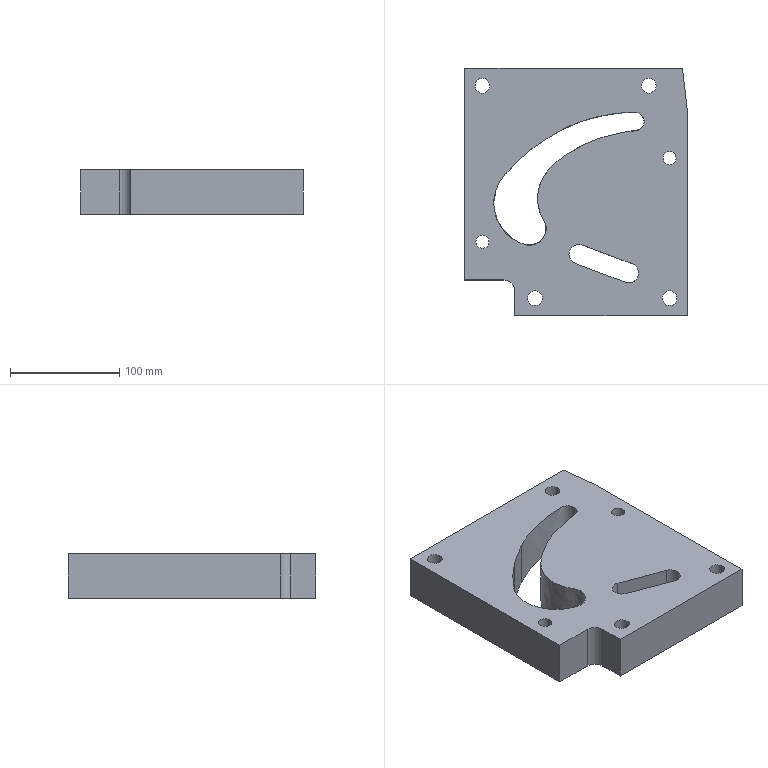Part | NX | features 7 2 | 1 solid | 90 faces | box 203 x 226 x 41 mm | volume 1435866 mm3 | plane 39 | cylinder 37 | cone 8 | spline 6 | commonest cylinder face diameters 10 x14 6.799 x8 20 x5 13.5 x4 12.001 x2 14.11 x2